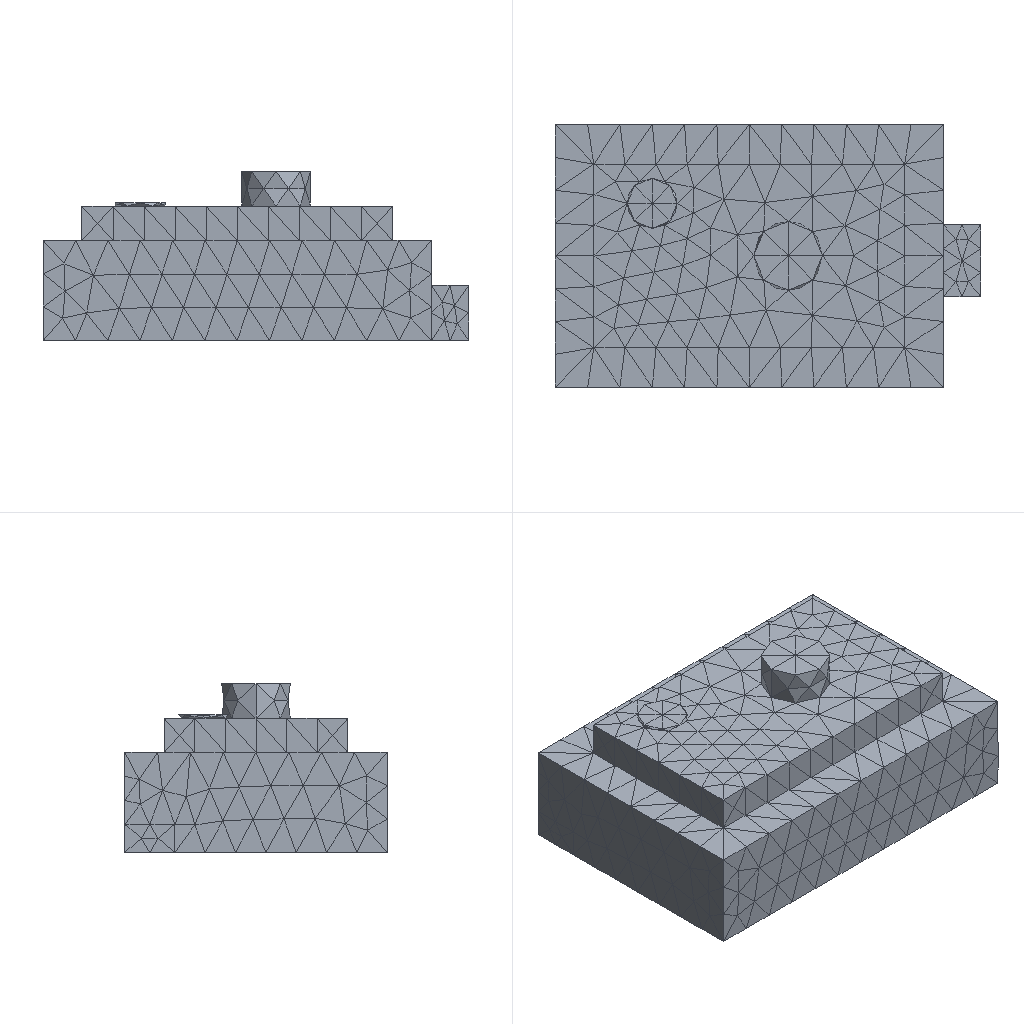Simulation study | ansys mapdl
Set-up summary:
category,name,step,type,value,unit,region
solver,ansys_mapdl
units,mm-N-s-tonne (MPa),,inferred,E=210000 density=
analysis,model,,static
mesh,nodes,,,5470
mesh,elements,,,3321
element_type,SOLID187,,,3321
material,mat 1,,E,210000
material,mat 1,,nu,0.3
load,,model,body load temp,,,all
load,,model,force,"1000 [dir=(0, 0, -1) n=95]",,node list
bc,,model,fixed,"[dofs=UX,UY,UZ n=5896]",,node list
Ansys APDL input file, long lists of numbers shortened:
/COM,ANSYS RELEASE 2026 R1           BUILD 26.1      UP20260202       09:09:04
/PREP7
/NOPR
/TITLE,2
ANTYPE, 0
*IF,_CDRDOFF,EQ,1,THEN     !if solid model was read in
_CDRDOFF=             !reset flag, numoffs already performed
*ELSE              !offset database for the following FE model
NUMOFF,NODE,     5470
NUMOFF,ELEM,     3321
NUMOFF,MAT ,        1
NUMOFF,TYPE,        1
*ENDIF
*SET,_RETURN ,  0.
*SET,_STATUS ,  0.
*SET,_UIQR   ,  95.
*SET,__FLOATPARAMETER__,  5470.
DOF,DELETE
ETBLOCK,        1,        1
(2i9,19a9)
        1      187        0        0        0        0        0        0        0        0        0        0        0        0        0        0        0        0        0        0        0
       -1
NBLOCK,6,SOLID,      5470,      5470
(3i9,6e21.13e3)
        1        0        0-4.6150000000000E+001 4.2000000000000E+001 9.0000000000000E+000
! (5469 more lines like these left out)
N,UNBL,LOC,       -1,
EBLOCK,19,SOLID,      3321,      3321
(19i10)
         1         1         1         1         0         0         0         0        10         0         1      1987      1988      1989      1990      2316      2317      2318      2319
! (6641 more lines like these left out)
        -1
MPTEMP,UNBL, 1, 1,  0.    ,
MPDATA,UNBL, 1,EX  ,       1, 1,  210000.000    ,
MPTEMP,UNBL, 1, 1,  0.    ,
MPDATA,UNBL, 1,NUXY,       1, 1, 0.3    ,
MPTEMP,UNBL, 1, 1,  0.    ,
MPDATA,UNBL, 1,PRXY,       1, 1, 0.3    ,
EXTOPT,ATTR,      0,      0,      0
EXTOPT,ESIZE,  0,  0.
EXTOPT,ACLEAR,      0
TREF,  0.
IRLF,  0
BFUNIF,TEMP,_TINY
ACEL,  0.    ,  0.    ,  0.
OMEGA,  0.    ,  0.    ,  0.
DOMEGA,  0.    ,  0.    ,  0.
CGLOC,  0.    ,  0.    ,  0.
CGOMEGA,  0.    ,  0.    ,  0.
DCGOMG,  0.    ,  0.    ,  0.
KUSE,     0
TIME,  0.
ALPHAD,  0.
BETAD,  0.
DMPRAT,  0.
DMPSTR,  0.
CRPLIM, 0.1    ,   0
CRPLIM,  0.    ,   1
NCNV,     0, 1.000000000E+12,     0,  0.    ,  0.
NEQIT,     0
ERESX,DEFA
DBLOCK,      5896
(i9,a6,2(pg16.9))
        1  UX    0.00000000      0.00000000
! (5895 more lines like these left out)
       -1
FBLOCK,        95
(i9,a6,2(pg16.9))
      966  FZ   -10.5263158      0.00000000
! (94 more lines like these left out)
       -1
/GO
FINISH
Results summary:
result,analysis_type_db,,,static,unstated
result,n_sets,,,1,unstated
result,load_steps[0].set,load_step=1,,1,unstated
result,load_steps[0].substep,load_step=1,,1,unstated
result,load_steps[0].time,load_step=1,,1,unstated
result,load_steps[0].freq,load_step=1,,1,unstated
result,load_steps[0].max_usum,load_step=1,,0.0002845,unstated
result,load_steps[0].max_seqv,load_step=1,,2.777,unstated
result,load_steps[0].reaction_sum.FX,load_step=1,,1.68732e-11,unstated
result,load_steps[0].reaction_sum.FY,load_step=1,,-8.11656e-12,unstated
result,load_steps[0].reaction_sum.FZ,load_step=1,,1000,unstated
result,load_steps[0].reaction_sum.MX,load_step=1,,0,unstated
result,load_steps[0].reaction_sum.MY,load_step=1,,0,unstated
result,load_steps[0].reaction_sum.MZ,load_step=1,,0,unstated
result,convergence,,,results present for all listed sets,unstated